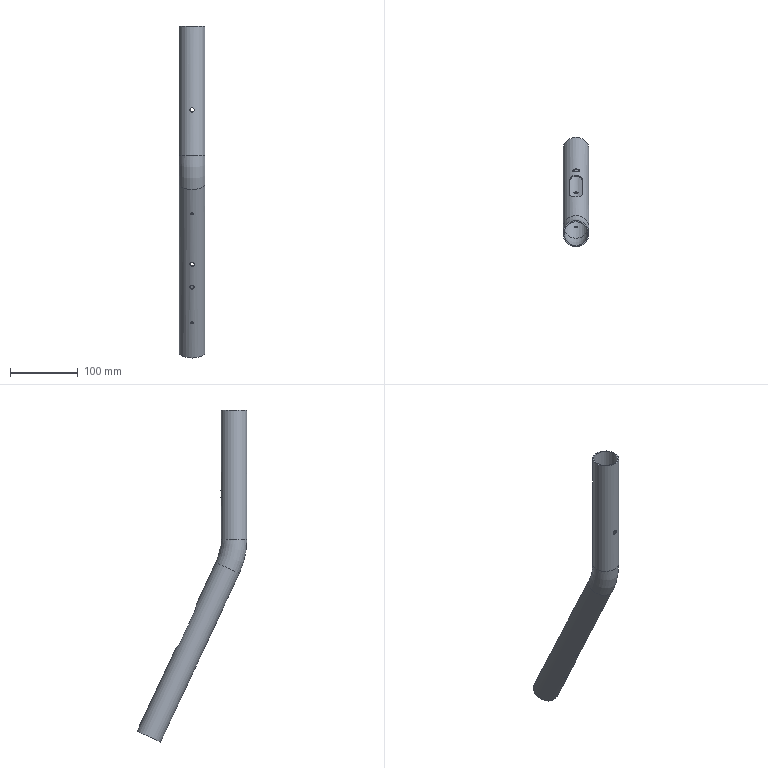Part | STEP file | Q7C1205L | 1 solid | 19 faces | box 38.1 x 161.362 x 488.383 mm | volume 85140 mm3 | cylinder 13 | plane 4 | torus 2 | commonest cylinder face diameters 6.5 x3 3.5 x2 10 x2 18 x2 35.1 x2 38.1 x2